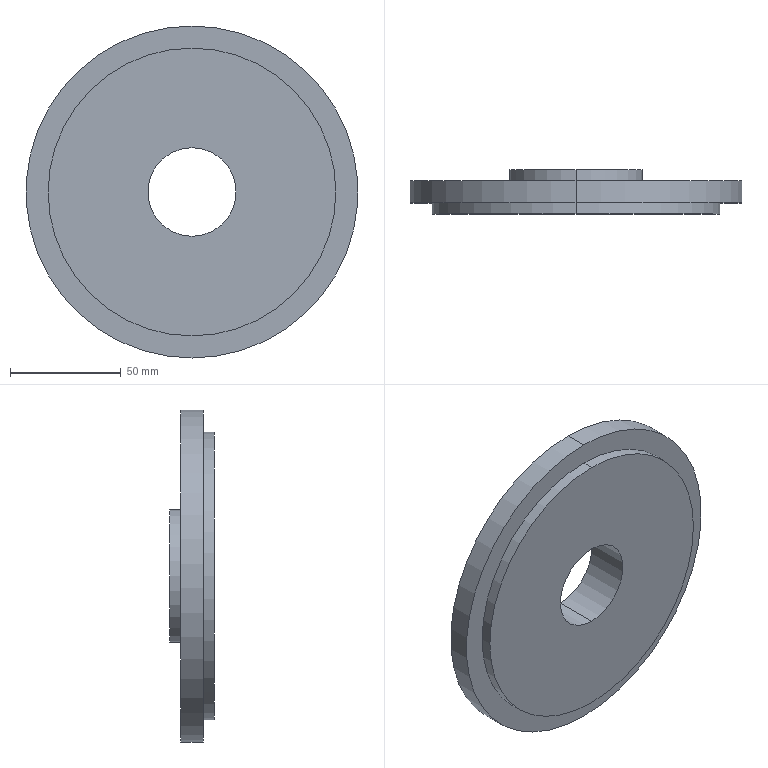Part | SolidWorks | 1 solid | 12 faces | box 150 x 20 x 150 mm | volume 232085 mm3 | cylinder 8 | plane 4 | commonest cylinder face diameters 40 x2 60 x2 130 x2 150 x2
STEP:
#1=CARTESIAN_POINT('',(0.,5.,-65.));
#2=VERTEX_POINT('',#1);
#3=CARTESIAN_POINT('',(0.,5.,65.));
#4=VERTEX_POINT('',#3);
#5=CARTESIAN_POINT('',(0.,5.,0.));
#6=DIRECTION('',(0.,-1.,0.));
#7=DIRECTION('',(0.,0.,-1.));
#8=AXIS2_PLACEMENT_3D('',#5,#6,#7);
#9=CIRCLE('',#8,65.);
#10=EDGE_CURVE('',#2,#4,#9,.T.);
#11=ORIENTED_EDGE('',*,*,#10,.T.);
#12=CARTESIAN_POINT('',(0.,0.,65.));
#13=VERTEX_POINT('',#12);
#14=CARTESIAN_POINT('',(0.,5.,65.));
#15=DIRECTION('',(0.,-1.,0.));
#16=VECTOR('',#15,1000.);
#17=LINE('',#14,#16);
#18=EDGE_CURVE('',#4,#13,#17,.T.);
#19=ORIENTED_EDGE('',*,*,#18,.T.);
#20=CARTESIAN_POINT('',(0.,0.,-65.));
#21=VERTEX_POINT('',#20);
#22=CARTESIAN_POINT('',(0.,0.,0.));
#23=DIRECTION('',(0.,-1.,0.));
#24=DIRECTION('',(0.,0.,-1.));
#25=AXIS2_PLACEMENT_3D('',#22,#23,#24);
#26=CIRCLE('',#25,65.);
#27=EDGE_CURVE('',#21,#13,#26,.T.);
#28=ORIENTED_EDGE('',*,*,#27,.F.);
#29=CARTESIAN_POINT('',(0.,5.,-65.));
#30=DIRECTION('',(0.,-1.,0.));
#31=VECTOR('',#30,1000.);
#32=LINE('',#29,#31);
#33=EDGE_CURVE('',#2,#21,#32,.T.);
#34=ORIENTED_EDGE('',*,*,#33,.F.);
#35=EDGE_LOOP('',(#11,#19,#28,#34));
#36=FACE_OUTER_BOUND('',#35,.T.);
#37=CARTESIAN_POINT('',(0.,5.,0.));
#38=DIRECTION('',(0.,-1.,0.));
#39=DIRECTION('',(0.,0.,-1.));
#40=AXIS2_PLACEMENT_3D('',#37,#38,#39);
#41=CYLINDRICAL_SURFACE('',#40,65.);
#42=ADVANCED_FACE('',(#36),#41,.T.);
#43=CARTESIAN_POINT('',(0.,0.,20.));
#44=VERTEX_POINT('',#43);
#45=CARTESIAN_POINT('',(0.,0.,-20.));
#46=VERTEX_POINT('',#45);
#47=CARTESIAN_POINT('',(0.,0.,0.));
#48=DIRECTION('',(0.,-1.,0.));
#49=DIRECTION('',(0.,0.,-1.));
#50=AXIS2_PLACEMENT_3D('',#47,#48,#49);
#51=CIRCLE('',#50,20.);
#52=EDGE_CURVE('',#44,#46,#51,.T.);
#53=ORIENTED_EDGE('',*,*,#52,.T.);
#54=CARTESIAN_POINT('',(0.,20.,-20.));
#55=VERTEX_POINT('',#54);
#56=CARTESIAN_POINT('',(0.,-58.,-20.));
#57=DIRECTION('',(0.,1.,0.));
#58=VECTOR('',#57,1000.);
#59=LINE('',#56,#58);
#60=EDGE_CURVE('',#46,#55,#59,.T.);
#61=ORIENTED_EDGE('',*,*,#60,.T.);
#62=CARTESIAN_POINT('',(0.,20.,20.));
#63=VERTEX_POINT('',#62);
#64=CARTESIAN_POINT('',(0.,20.,0.));
#65=DIRECTION('',(0.,1.,0.));
#66=DIRECTION('',(0.,0.,1.));
#67=AXIS2_PLACEMENT_3D('',#64,#65,#66);
#68=CIRCLE('',#67,20.);
#69=EDGE_CURVE('',#55,#63,#68,.T.);
#70=ORIENTED_EDGE('',*,*,#69,.T.);
#71=CARTESIAN_POINT('',(0.,-58.,20.));
#72=DIRECTION('',(0.,1.,0.));
#73=VECTOR('',#72,1000.);
#74=LINE('',#71,#73);
#75=EDGE_CURVE('',#44,#63,#74,.T.);
#76=ORIENTED_EDGE('',*,*,#75,.F.);
#77=EDGE_LOOP('',(#53,#61,#70,#76));
#78=FACE_OUTER_BOUND('',#77,.T.);
#79=CARTESIAN_POINT('',(0.,-58.,0.));
#80=DIRECTION('',(0.,1.,0.));
#81=DIRECTION('',(0.,0.,1.));
#82=AXIS2_PLACEMENT_3D('',#79,#80,#81);
#83=CYLINDRICAL_SURFACE('',#82,20.);
#84=ADVANCED_FACE('',(#78),#83,.F.);
#85=CARTESIAN_POINT('',(0.,20.,-30.));
#86=VERTEX_POINT('',#85);
#87=CARTESIAN_POINT('',(0.,20.,30.));
#88=VERTEX_POINT('',#87);
#89=CARTESIAN_POINT('',(0.,20.,0.));
#90=DIRECTION('',(0.,-1.,0.));
#91=DIRECTION('',(0.,0.,-1.));
#92=AXIS2_PLACEMENT_3D('',#89,#90,#91);
#93=CIRCLE('',#92,30.);
#94=EDGE_CURVE('',#86,#88,#93,.T.);
#95=ORIENTED_EDGE('',*,*,#94,.T.);
#96=CARTESIAN_POINT('',(0.,15.,30.));
#97=VERTEX_POINT('',#96);
#98=CARTESIAN_POINT('',(0.,0.,30.));
#99=DIRECTION('',(0.,-1.,0.));
#100=VECTOR('',#99,1000.);
#101=LINE('',#98,#100);
#102=EDGE_CURVE('',#88,#97,#101,.T.);
#103=ORIENTED_EDGE('',*,*,#102,.T.);
#104=CARTESIAN_POINT('',(0.,15.,-30.));
#105=VERTEX_POINT('',#104);
#106=CARTESIAN_POINT('',(0.,15.,0.));
#107=DIRECTION('',(0.,-1.,0.));
#108=DIRECTION('',(0.,0.,-1.));
#109=AXIS2_PLACEMENT_3D('',#106,#107,#108);
#110=CIRCLE('',#109,30.);
#111=EDGE_CURVE('',#105,#97,#110,.T.);
#112=ORIENTED_EDGE('',*,*,#111,.F.);
#113=CARTESIAN_POINT('',(0.,0.,-30.));
#114=DIRECTION('',(0.,-1.,0.));
#115=VECTOR('',#114,1000.);
#116=LINE('',#113,#115);
#117=EDGE_CURVE('',#86,#105,#116,.T.);
#118=ORIENTED_EDGE('',*,*,#117,.F.);
#119=EDGE_LOOP('',(#95,#103,#112,#118));
#120=FACE_OUTER_BOUND('',#119,.T.);
#121=CARTESIAN_POINT('',(0.,0.,0.));
#122=DIRECTION('',(0.,-1.,0.));
#123=DIRECTION('',(0.,0.,-1.));
#124=AXIS2_PLACEMENT_3D('',#121,#122,#123);
#125=CYLINDRICAL_SURFACE('',#124,30.);
#126=ADVANCED_FACE('',(#120),#125,.T.);
#127=CARTESIAN_POINT('',(0.,15.,-75.));
#128=VERTEX_POINT('',#127);
#129=CARTESIAN_POINT('',(0.,15.,75.));
#130=VERTEX_POINT('',#129);
#131=CARTESIAN_POINT('',(0.,15.,0.));
#132=DIRECTION('',(0.,-1.,0.));
#133=DIRECTION('',(0.,0.,-1.));
#134=AXIS2_PLACEMENT_3D('',#131,#132,#133);
#135=CIRCLE('',#134,75.);
#136=EDGE_CURVE('',#128,#130,#135,.T.);
#137=ORIENTED_EDGE('',*,*,#136,.T.);
#138=CARTESIAN_POINT('',(0.,5.,75.));
#139=VERTEX_POINT('',#138);
#140=CARTESIAN_POINT('',(0.,0.,75.));
#141=DIRECTION('',(0.,-1.,0.));
#142=VECTOR('',#141,1000.);
#143=LINE('',#140,#142);
#144=EDGE_CURVE('',#130,#139,#143,.T.);
#145=ORIENTED_EDGE('',*,*,#144,.T.);
#146=CARTESIAN_POINT('',(0.,5.,-75.));
#147=VERTEX_POINT('',#146);
#148=CARTESIAN_POINT('',(0.,5.,0.));
#149=DIRECTION('',(0.,1.,0.));
#150=DIRECTION('',(0.,0.,-1.));
#151=AXIS2_PLACEMENT_3D('',#148,#149,#150);
#152=CIRCLE('',#151,75.);
#153=EDGE_CURVE('',#139,#147,#152,.T.);
#154=ORIENTED_EDGE('',*,*,#153,.T.);
#155=CARTESIAN_POINT('',(0.,0.,-75.));
#156=DIRECTION('',(0.,-1.,0.));
#157=VECTOR('',#156,1000.);
#158=LINE('',#155,#157);
#159=EDGE_CURVE('',#128,#147,#158,.T.);
#160=ORIENTED_EDGE('',*,*,#159,.F.);
#161=EDGE_LOOP('',(#137,#145,#154,#160));
#162=FACE_OUTER_BOUND('',#161,.T.);
#163=CARTESIAN_POINT('',(0.,0.,0.));
#164=DIRECTION('',(0.,-1.,0.));
#165=DIRECTION('',(0.,0.,-1.));
#166=AXIS2_PLACEMENT_3D('',#163,#164,#165);
#167=CYLINDRICAL_SURFACE('',#166,75.);
#168=ADVANCED_FACE('',(#162),#167,.T.);
#169=ORIENTED_EDGE('',*,*,#144,.F.);
#170=CARTESIAN_POINT('',(0.,15.,0.));
#171=DIRECTION('',(0.,-1.,0.));
#172=DIRECTION('',(0.,0.,-1.));
#173=AXIS2_PLACEMENT_3D('',#170,#171,#172);
#174=CIRCLE('',#173,75.);
#175=EDGE_CURVE('',#130,#128,#174,.T.);
#176=ORIENTED_EDGE('',*,*,#175,.T.);
#177=ORIENTED_EDGE('',*,*,#159,.T.);
#178=CARTESIAN_POINT('',(0.,5.,0.));
#179=DIRECTION('',(0.,1.,0.));
#180=DIRECTION('',(0.,0.,-1.));
#181=AXIS2_PLACEMENT_3D('',#178,#179,#180);
#182=CIRCLE('',#181,75.);
#183=EDGE_CURVE('',#147,#139,#182,.T.);
#184=ORIENTED_EDGE('',*,*,#183,.T.);
#185=EDGE_LOOP('',(#169,#176,#177,#184));
#186=FACE_OUTER_BOUND('',#185,.T.);
#187=CARTESIAN_POINT('',(0.,0.,0.));
#188=DIRECTION('',(0.,-1.,0.));
#189=DIRECTION('',(0.,0.,-1.));
#190=AXIS2_PLACEMENT_3D('',#187,#188,#189);
#191=CYLINDRICAL_SURFACE('',#190,75.);
#192=ADVANCED_FACE('',(#186),#191,.T.);
#193=ORIENTED_EDGE('',*,*,#52,.F.);
#194=CARTESIAN_POINT('',(0.,0.,0.));
#195=DIRECTION('',(0.,-1.,0.));
#196=DIRECTION('',(0.,0.,-1.));
#197=AXIS2_PLACEMENT_3D('',#194,#195,#196);
#198=CIRCLE('',#197,20.);
#199=EDGE_CURVE('',#46,#44,#198,.T.);
#200=ORIENTED_EDGE('',*,*,#199,.F.);
#201=EDGE_LOOP('',(#193,#200));
#202=FACE_BOUND('',#201,.T.);
#203=ORIENTED_EDGE('',*,*,#27,.T.);
#204=CARTESIAN_POINT('',(0.,0.,0.));
#205=DIRECTION('',(0.,-1.,0.));
#206=DIRECTION('',(0.,0.,-1.));
#207=AXIS2_PLACEMENT_3D('',#204,#205,#206);
#208=CIRCLE('',#207,65.);
#209=EDGE_CURVE('',#13,#21,#208,.T.);
#210=ORIENTED_EDGE('',*,*,#209,.T.);
#211=EDGE_LOOP('',(#203,#210));
#212=FACE_OUTER_BOUND('',#211,.T.);
#213=CARTESIAN_POINT('',(75.,0.,0.));
#214=DIRECTION('',(0.,-1.,0.));
#215=DIRECTION('',(0.,0.,-1.));
#216=AXIS2_PLACEMENT_3D('',#213,#214,#215);
#217=PLANE('',#216);
#218=ADVANCED_FACE('',(#202,#212),#217,.T.);
#219=CARTESIAN_POINT('',(0.,20.,0.));
#220=DIRECTION('',(0.,1.,0.));
#221=DIRECTION('',(0.,0.,1.));
#222=AXIS2_PLACEMENT_3D('',#219,#220,#221);
#223=CIRCLE('',#222,20.);
#224=EDGE_CURVE('',#63,#55,#223,.T.);
#225=ORIENTED_EDGE('',*,*,#224,.F.);
#226=ORIENTED_EDGE('',*,*,#69,.F.);
#227=EDGE_LOOP('',(#225,#226));
#228=FACE_BOUND('',#227,.T.);
#229=ORIENTED_EDGE('',*,*,#94,.F.);
#230=CARTESIAN_POINT('',(0.,20.,0.));
#231=DIRECTION('',(0.,-1.,0.));
#232=DIRECTION('',(0.,0.,-1.));
#233=AXIS2_PLACEMENT_3D('',#230,#231,#232);
#234=CIRCLE('',#233,30.);
#235=EDGE_CURVE('',#88,#86,#234,.T.);
#236=ORIENTED_EDGE('',*,*,#235,.F.);
#237=EDGE_LOOP('',(#229,#236));
#238=FACE_OUTER_BOUND('',#237,.T.);
#239=CARTESIAN_POINT('',(0.,20.,0.));
#240=DIRECTION('',(0.,1.,0.));
#241=DIRECTION('',(0.,0.,1.));
#242=AXIS2_PLACEMENT_3D('',#239,#240,#241);
#243=PLANE('',#242);
#244=ADVANCED_FACE('',(#228,#238),#243,.T.);
#245=ORIENTED_EDGE('',*,*,#102,.F.);
#246=ORIENTED_EDGE('',*,*,#235,.T.);
#247=ORIENTED_EDGE('',*,*,#117,.T.);
#248=CARTESIAN_POINT('',(0.,15.,0.));
#249=DIRECTION('',(0.,-1.,0.));
#250=DIRECTION('',(0.,0.,-1.));
#251=AXIS2_PLACEMENT_3D('',#248,#249,#250);
#252=CIRCLE('',#251,30.);
#253=EDGE_CURVE('',#97,#105,#252,.T.);
#254=ORIENTED_EDGE('',*,*,#253,.F.);
#255=EDGE_LOOP('',(#245,#246,#247,#254));
#256=FACE_OUTER_BOUND('',#255,.T.);
#257=CARTESIAN_POINT('',(0.,0.,0.));
#258=DIRECTION('',(0.,-1.,0.));
#259=DIRECTION('',(0.,0.,-1.));
#260=AXIS2_PLACEMENT_3D('',#257,#258,#259);
#261=CYLINDRICAL_SURFACE('',#260,30.);
#262=ADVANCED_FACE('',(#256),#261,.T.);
#263=ORIENTED_EDGE('',*,*,#111,.T.);
#264=ORIENTED_EDGE('',*,*,#253,.T.);
#265=EDGE_LOOP('',(#263,#264));
#266=FACE_BOUND('',#265,.T.);
#267=ORIENTED_EDGE('',*,*,#136,.F.);
#268=ORIENTED_EDGE('',*,*,#175,.F.);
#269=EDGE_LOOP('',(#267,#268));
#270=FACE_OUTER_BOUND('',#269,.T.);
#271=CARTESIAN_POINT('',(30.,15.,0.));
#272=DIRECTION('',(0.,1.,0.));
#273=DIRECTION('',(0.,0.,1.));
#274=AXIS2_PLACEMENT_3D('',#271,#272,#273);
#275=PLANE('',#274);
#276=ADVANCED_FACE('',(#266,#270),#275,.T.);
#277=ORIENTED_EDGE('',*,*,#60,.F.);
#278=ORIENTED_EDGE('',*,*,#199,.T.);
#279=ORIENTED_EDGE('',*,*,#75,.T.);
#280=ORIENTED_EDGE('',*,*,#224,.T.);
#281=EDGE_LOOP('',(#277,#278,#279,#280));
#282=FACE_OUTER_BOUND('',#281,.T.);
#283=CARTESIAN_POINT('',(0.,-58.,0.));
#284=DIRECTION('',(0.,1.,0.));
#285=DIRECTION('',(0.,0.,1.));
#286=AXIS2_PLACEMENT_3D('',#283,#284,#285);
#287=CYLINDRICAL_SURFACE('',#286,20.);
#288=ADVANCED_FACE('',(#282),#287,.F.);
#289=ORIENTED_EDGE('',*,*,#183,.F.);
#290=ORIENTED_EDGE('',*,*,#153,.F.);
#291=EDGE_LOOP('',(#289,#290));
#292=FACE_OUTER_BOUND('',#291,.T.);
#293=ORIENTED_EDGE('',*,*,#10,.F.);
#294=CARTESIAN_POINT('',(0.,5.,0.));
#295=DIRECTION('',(0.,-1.,0.));
#296=DIRECTION('',(0.,0.,-1.));
#297=AXIS2_PLACEMENT_3D('',#294,#295,#296);
#298=CIRCLE('',#297,65.);
#299=EDGE_CURVE('',#4,#2,#298,.T.);
#300=ORIENTED_EDGE('',*,*,#299,.F.);
#301=EDGE_LOOP('',(#293,#300));
#302=FACE_BOUND('',#301,.T.);
#303=CARTESIAN_POINT('',(0.,5.,0.));
#304=DIRECTION('',(0.,-1.,0.));
#305=DIRECTION('',(0.,0.,-1.));
#306=AXIS2_PLACEMENT_3D('',#303,#304,#305);
#307=PLANE('',#306);
#308=ADVANCED_FACE('',(#292,#302),#307,.T.);
#309=ORIENTED_EDGE('',*,*,#18,.F.);
#310=ORIENTED_EDGE('',*,*,#299,.T.);
#311=ORIENTED_EDGE('',*,*,#33,.T.);
#312=ORIENTED_EDGE('',*,*,#209,.F.);
#313=EDGE_LOOP('',(#309,#310,#311,#312));
#314=FACE_OUTER_BOUND('',#313,.T.);
#315=CARTESIAN_POINT('',(0.,5.,0.));
#316=DIRECTION('',(0.,-1.,0.));
#317=DIRECTION('',(0.,0.,-1.));
#318=AXIS2_PLACEMENT_3D('',#315,#316,#317);
#319=CYLINDRICAL_SURFACE('',#318,65.);
#320=ADVANCED_FACE('',(#314),#319,.T.);
#321=CLOSED_SHELL('',(#42,#84,#126,#168,#192,#218,#244,#262,#276,#288,#308,#320));
#322=MANIFOLD_SOLID_BREP('',#321);
#323=CARTESIAN_POINT('',(0.,0.,0.));
#324=DIRECTION('',(0.,0.,1.));
#325=DIRECTION('',(1.,0.,0.));
#326=AXIS2_PLACEMENT_3D('',#323,#324,#325);
#327=(LENGTH_UNIT()NAMED_UNIT(*)SI_UNIT(.MILLI.,.METRE.));
#328=UNCERTAINTY_MEASURE_WITH_UNIT(LENGTH_MEASURE(0.00001),#327,'','');
#329=(NAMED_UNIT(*)PLANE_ANGLE_UNIT()SI_UNIT($,.RADIAN.));
#330=(NAMED_UNIT(*)SI_UNIT($,.STERADIAN.)SOLID_ANGLE_UNIT());
#331=(GEOMETRIC_REPRESENTATION_CONTEXT(3)GLOBAL_UNCERTAINTY_ASSIGNED_CONTEXT((#328))GLOBAL_UNIT_ASSIGNED_CONTEXT((#327,#329,#330))REPRESENTATION_CONTEXT('',''));
#332=ADVANCED_BREP_SHAPE_REPRESENTATION('',(#322,#326),#331);